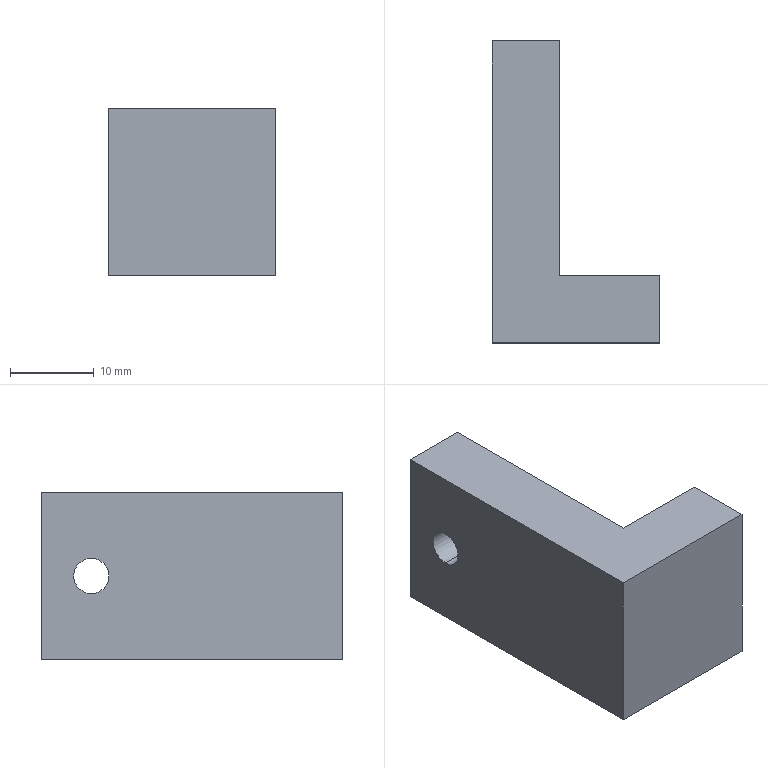Part | SolidWorks | features 3DProfileFeature 1, Extrusion 1, HoleWzd 1 | 1 solid | 10 faces | box 20 x 36 x 20 mm | volume 7569 mm3 | plane 8 | cylinder 2 | commonest cylinder face diameters 4.2 x2
STEP:
#1=CARTESIAN_POINT('',(-12.,30.,-2.1));
#2=VERTEX_POINT('',#1);
#3=CARTESIAN_POINT('',(-12.,30.,2.1));
#4=VERTEX_POINT('',#3);
#5=CARTESIAN_POINT('',(-12.,30.,0.));
#6=DIRECTION('',(-1.,0.,0.));
#7=DIRECTION('',(0.,0.,1.));
#8=AXIS2_PLACEMENT_3D('',#5,#6,#7);
#9=CIRCLE('',#8,2.1);
#10=EDGE_CURVE('',#2,#4,#9,.T.);
#11=ORIENTED_EDGE('',*,*,#10,.F.);
#12=CARTESIAN_POINT('',(-20.,30.,-2.1));
#13=VERTEX_POINT('',#12);
#14=CARTESIAN_POINT('',(-20.,30.,-2.1));
#15=DIRECTION('',(-1.,0.,0.));
#16=VECTOR('',#15,1000.);
#17=LINE('',#14,#16);
#18=EDGE_CURVE('',#2,#13,#17,.T.);
#19=ORIENTED_EDGE('',*,*,#18,.T.);
#20=CARTESIAN_POINT('',(-20.,30.,2.1));
#21=VERTEX_POINT('',#20);
#22=CARTESIAN_POINT('',(-20.,30.,0.));
#23=DIRECTION('',(-1.,0.,0.));
#24=DIRECTION('',(0.,0.,1.));
#25=AXIS2_PLACEMENT_3D('',#22,#23,#24);
#26=CIRCLE('',#25,2.1);
#27=EDGE_CURVE('',#13,#21,#26,.T.);
#28=ORIENTED_EDGE('',*,*,#27,.T.);
#29=CARTESIAN_POINT('',(-20.,30.,2.1));
#30=DIRECTION('',(-1.,0.,0.));
#31=VECTOR('',#30,1000.);
#32=LINE('',#29,#31);
#33=EDGE_CURVE('',#4,#21,#32,.T.);
#34=ORIENTED_EDGE('',*,*,#33,.F.);
#35=EDGE_LOOP('',(#11,#19,#28,#34));
#36=FACE_OUTER_BOUND('',#35,.T.);
#37=CARTESIAN_POINT('',(-20.,30.,0.));
#38=DIRECTION('',(-1.,0.,0.));
#39=DIRECTION('',(0.,0.,1.));
#40=AXIS2_PLACEMENT_3D('',#37,#38,#39);
#41=CYLINDRICAL_SURFACE('',#40,2.1);
#42=ADVANCED_FACE('',(#36),#41,.F.);
#43=CARTESIAN_POINT('',(-20.,36.,-10.));
#44=VERTEX_POINT('',#43);
#45=CARTESIAN_POINT('',(-20.,0.,-10.));
#46=VERTEX_POINT('',#45);
#47=CARTESIAN_POINT('',(-20.,0.,-10.));
#48=DIRECTION('',(0.,-1.,0.));
#49=VECTOR('',#48,1000.);
#50=LINE('',#47,#49);
#51=EDGE_CURVE('',#44,#46,#50,.T.);
#52=ORIENTED_EDGE('',*,*,#51,.T.);
#53=CARTESIAN_POINT('',(-20.,0.,10.));
#54=VERTEX_POINT('',#53);
#55=CARTESIAN_POINT('',(-20.,0.,10.));
#56=DIRECTION('',(0.,0.,-1.));
#57=VECTOR('',#56,1000.);
#58=LINE('',#55,#57);
#59=EDGE_CURVE('',#54,#46,#58,.T.);
#60=ORIENTED_EDGE('',*,*,#59,.F.);
#61=CARTESIAN_POINT('',(-20.,36.,10.));
#62=VERTEX_POINT('',#61);
#63=CARTESIAN_POINT('',(-20.,0.,10.));
#64=DIRECTION('',(0.,-1.,0.));
#65=VECTOR('',#64,1000.);
#66=LINE('',#63,#65);
#67=EDGE_CURVE('',#62,#54,#66,.T.);
#68=ORIENTED_EDGE('',*,*,#67,.F.);
#69=CARTESIAN_POINT('',(-20.,36.,10.));
#70=DIRECTION('',(0.,0.,-1.));
#71=VECTOR('',#70,1000.);
#72=LINE('',#69,#71);
#73=EDGE_CURVE('',#62,#44,#72,.T.);
#74=ORIENTED_EDGE('',*,*,#73,.T.);
#75=EDGE_LOOP('',(#52,#60,#68,#74));
#76=FACE_OUTER_BOUND('',#75,.T.);
#77=CARTESIAN_POINT('',(-20.,30.,0.));
#78=DIRECTION('',(-1.,0.,0.));
#79=DIRECTION('',(0.,0.,1.));
#80=AXIS2_PLACEMENT_3D('',#77,#78,#79);
#81=CIRCLE('',#80,2.1);
#82=EDGE_CURVE('',#21,#13,#81,.T.);
#83=ORIENTED_EDGE('',*,*,#82,.F.);
#84=ORIENTED_EDGE('',*,*,#27,.F.);
#85=EDGE_LOOP('',(#83,#84));
#86=FACE_BOUND('',#85,.T.);
#87=CARTESIAN_POINT('',(-20.,0.,10.));
#88=DIRECTION('',(1.,0.,0.));
#89=DIRECTION('',(0.,0.,-1.));
#90=AXIS2_PLACEMENT_3D('',#87,#88,#89);
#91=PLANE('',#90);
#92=ADVANCED_FACE('',(#76,#86),#91,.F.);
#93=CARTESIAN_POINT('',(0.,0.,-10.));
#94=VERTEX_POINT('',#93);
#95=CARTESIAN_POINT('',(0.,8.,-10.));
#96=VERTEX_POINT('',#95);
#97=CARTESIAN_POINT('',(0.,8.,-10.));
#98=DIRECTION('',(0.,1.,0.));
#99=VECTOR('',#98,1000.);
#100=LINE('',#97,#99);
#101=EDGE_CURVE('',#94,#96,#100,.T.);
#102=ORIENTED_EDGE('',*,*,#101,.T.);
#103=CARTESIAN_POINT('',(0.,8.,10.));
#104=VERTEX_POINT('',#103);
#105=CARTESIAN_POINT('',(0.,8.,10.));
#106=DIRECTION('',(0.,0.,-1.));
#107=VECTOR('',#106,1000.);
#108=LINE('',#105,#107);
#109=EDGE_CURVE('',#104,#96,#108,.T.);
#110=ORIENTED_EDGE('',*,*,#109,.F.);
#111=CARTESIAN_POINT('',(0.,0.,10.));
#112=VERTEX_POINT('',#111);
#113=CARTESIAN_POINT('',(0.,8.,10.));
#114=DIRECTION('',(0.,1.,0.));
#115=VECTOR('',#114,1000.);
#116=LINE('',#113,#115);
#117=EDGE_CURVE('',#112,#104,#116,.T.);
#118=ORIENTED_EDGE('',*,*,#117,.F.);
#119=CARTESIAN_POINT('',(0.,0.,10.));
#120=DIRECTION('',(0.,0.,-1.));
#121=VECTOR('',#120,1000.);
#122=LINE('',#119,#121);
#123=EDGE_CURVE('',#112,#94,#122,.T.);
#124=ORIENTED_EDGE('',*,*,#123,.T.);
#125=EDGE_LOOP('',(#102,#110,#118,#124));
#126=FACE_OUTER_BOUND('',#125,.T.);
#127=CARTESIAN_POINT('',(0.,8.,10.));
#128=DIRECTION('',(-1.,0.,0.));
#129=DIRECTION('',(0.,-1.,0.));
#130=AXIS2_PLACEMENT_3D('',#127,#128,#129);
#131=PLANE('',#130);
#132=ADVANCED_FACE('',(#126),#131,.F.);
#133=CARTESIAN_POINT('',(-12.,8.,-10.));
#134=VERTEX_POINT('',#133);
#135=CARTESIAN_POINT('',(-12.,8.,-10.));
#136=DIRECTION('',(-1.,0.,0.));
#137=VECTOR('',#136,1000.);
#138=LINE('',#135,#137);
#139=EDGE_CURVE('',#96,#134,#138,.T.);
#140=ORIENTED_EDGE('',*,*,#139,.T.);
#141=CARTESIAN_POINT('',(-12.,8.,10.));
#142=VERTEX_POINT('',#141);
#143=CARTESIAN_POINT('',(-12.,8.,10.));
#144=DIRECTION('',(0.,0.,-1.));
#145=VECTOR('',#144,1000.);
#146=LINE('',#143,#145);
#147=EDGE_CURVE('',#142,#134,#146,.T.);
#148=ORIENTED_EDGE('',*,*,#147,.F.);
#149=CARTESIAN_POINT('',(-12.,8.,10.));
#150=DIRECTION('',(-1.,0.,0.));
#151=VECTOR('',#150,1000.);
#152=LINE('',#149,#151);
#153=EDGE_CURVE('',#104,#142,#152,.T.);
#154=ORIENTED_EDGE('',*,*,#153,.F.);
#155=ORIENTED_EDGE('',*,*,#109,.T.);
#156=EDGE_LOOP('',(#140,#148,#154,#155));
#157=FACE_OUTER_BOUND('',#156,.T.);
#158=CARTESIAN_POINT('',(-12.,8.,10.));
#159=DIRECTION('',(0.,-1.,0.));
#160=DIRECTION('',(0.,0.,-1.));
#161=AXIS2_PLACEMENT_3D('',#158,#159,#160);
#162=PLANE('',#161);
#163=ADVANCED_FACE('',(#157),#162,.F.);
#164=CARTESIAN_POINT('',(-12.,30.,0.));
#165=DIRECTION('',(-1.,0.,0.));
#166=DIRECTION('',(0.,0.,1.));
#167=AXIS2_PLACEMENT_3D('',#164,#165,#166);
#168=CIRCLE('',#167,2.1);
#169=EDGE_CURVE('',#4,#2,#168,.T.);
#170=ORIENTED_EDGE('',*,*,#169,.T.);
#171=ORIENTED_EDGE('',*,*,#10,.T.);
#172=EDGE_LOOP('',(#170,#171));
#173=FACE_BOUND('',#172,.T.);
#174=CARTESIAN_POINT('',(-12.,36.,-10.));
#175=VERTEX_POINT('',#174);
#176=CARTESIAN_POINT('',(-12.,36.,-10.));
#177=DIRECTION('',(0.,1.,0.));
#178=VECTOR('',#177,1000.);
#179=LINE('',#176,#178);
#180=EDGE_CURVE('',#134,#175,#179,.T.);
#181=ORIENTED_EDGE('',*,*,#180,.T.);
#182=CARTESIAN_POINT('',(-12.,36.,10.));
#183=VERTEX_POINT('',#182);
#184=CARTESIAN_POINT('',(-12.,36.,10.));
#185=DIRECTION('',(0.,0.,-1.));
#186=VECTOR('',#185,1000.);
#187=LINE('',#184,#186);
#188=EDGE_CURVE('',#183,#175,#187,.T.);
#189=ORIENTED_EDGE('',*,*,#188,.F.);
#190=CARTESIAN_POINT('',(-12.,36.,10.));
#191=DIRECTION('',(0.,1.,0.));
#192=VECTOR('',#191,1000.);
#193=LINE('',#190,#192);
#194=EDGE_CURVE('',#142,#183,#193,.T.);
#195=ORIENTED_EDGE('',*,*,#194,.F.);
#196=ORIENTED_EDGE('',*,*,#147,.T.);
#197=EDGE_LOOP('',(#181,#189,#195,#196));
#198=FACE_OUTER_BOUND('',#197,.T.);
#199=CARTESIAN_POINT('',(-12.,36.,10.));
#200=DIRECTION('',(-1.,0.,0.));
#201=DIRECTION('',(0.,0.,1.));
#202=AXIS2_PLACEMENT_3D('',#199,#200,#201);
#203=PLANE('',#202);
#204=ADVANCED_FACE('',(#173,#198),#203,.F.);
#205=CARTESIAN_POINT('',(-20.,36.,-10.));
#206=DIRECTION('',(-1.,0.,0.));
#207=VECTOR('',#206,1000.);
#208=LINE('',#205,#207);
#209=EDGE_CURVE('',#175,#44,#208,.T.);
#210=ORIENTED_EDGE('',*,*,#209,.T.);
#211=ORIENTED_EDGE('',*,*,#73,.F.);
#212=CARTESIAN_POINT('',(-20.,36.,10.));
#213=DIRECTION('',(-1.,0.,0.));
#214=VECTOR('',#213,1000.);
#215=LINE('',#212,#214);
#216=EDGE_CURVE('',#183,#62,#215,.T.);
#217=ORIENTED_EDGE('',*,*,#216,.F.);
#218=ORIENTED_EDGE('',*,*,#188,.T.);
#219=EDGE_LOOP('',(#210,#211,#217,#218));
#220=FACE_OUTER_BOUND('',#219,.T.);
#221=CARTESIAN_POINT('',(-20.,36.,10.));
#222=DIRECTION('',(0.,-1.,0.));
#223=DIRECTION('',(0.,0.,-1.));
#224=AXIS2_PLACEMENT_3D('',#221,#222,#223);
#225=PLANE('',#224);
#226=ADVANCED_FACE('',(#220),#225,.F.);
#227=CARTESIAN_POINT('',(0.,0.,-10.));
#228=DIRECTION('',(1.,0.,0.));
#229=VECTOR('',#228,1000.);
#230=LINE('',#227,#229);
#231=EDGE_CURVE('',#46,#94,#230,.T.);
#232=ORIENTED_EDGE('',*,*,#231,.T.);
#233=ORIENTED_EDGE('',*,*,#123,.F.);
#234=CARTESIAN_POINT('',(0.,0.,10.));
#235=DIRECTION('',(1.,0.,0.));
#236=VECTOR('',#235,1000.);
#237=LINE('',#234,#236);
#238=EDGE_CURVE('',#54,#112,#237,.T.);
#239=ORIENTED_EDGE('',*,*,#238,.F.);
#240=ORIENTED_EDGE('',*,*,#59,.T.);
#241=EDGE_LOOP('',(#232,#233,#239,#240));
#242=FACE_OUTER_BOUND('',#241,.T.);
#243=CARTESIAN_POINT('',(0.,0.,10.));
#244=DIRECTION('',(0.,1.,0.));
#245=DIRECTION('',(-1.,0.,0.));
#246=AXIS2_PLACEMENT_3D('',#243,#244,#245);
#247=PLANE('',#246);
#248=ADVANCED_FACE('',(#242),#247,.F.);
#249=ORIENTED_EDGE('',*,*,#117,.T.);
#250=ORIENTED_EDGE('',*,*,#153,.T.);
#251=ORIENTED_EDGE('',*,*,#194,.T.);
#252=ORIENTED_EDGE('',*,*,#216,.T.);
#253=ORIENTED_EDGE('',*,*,#67,.T.);
#254=ORIENTED_EDGE('',*,*,#238,.T.);
#255=EDGE_LOOP('',(#249,#250,#251,#252,#253,#254));
#256=FACE_OUTER_BOUND('',#255,.T.);
#257=CARTESIAN_POINT('',(0.,0.,10.));
#258=DIRECTION('',(0.,0.,-1.));
#259=DIRECTION('',(-1.,0.,0.));
#260=AXIS2_PLACEMENT_3D('',#257,#258,#259);
#261=PLANE('',#260);
#262=ADVANCED_FACE('',(#256),#261,.F.);
#263=ORIENTED_EDGE('',*,*,#101,.F.);
#264=ORIENTED_EDGE('',*,*,#231,.F.);
#265=ORIENTED_EDGE('',*,*,#51,.F.);
#266=ORIENTED_EDGE('',*,*,#209,.F.);
#267=ORIENTED_EDGE('',*,*,#180,.F.);
#268=ORIENTED_EDGE('',*,*,#139,.F.);
#269=EDGE_LOOP('',(#263,#264,#265,#266,#267,#268));
#270=FACE_OUTER_BOUND('',#269,.T.);
#271=CARTESIAN_POINT('',(0.,0.,-10.));
#272=DIRECTION('',(0.,0.,-1.));
#273=DIRECTION('',(-1.,0.,0.));
#274=AXIS2_PLACEMENT_3D('',#271,#272,#273);
#275=PLANE('',#274);
#276=ADVANCED_FACE('',(#270),#275,.T.);
#277=ORIENTED_EDGE('',*,*,#18,.F.);
#278=ORIENTED_EDGE('',*,*,#169,.F.);
#279=ORIENTED_EDGE('',*,*,#33,.T.);
#280=ORIENTED_EDGE('',*,*,#82,.T.);
#281=EDGE_LOOP('',(#277,#278,#279,#280));
#282=FACE_OUTER_BOUND('',#281,.T.);
#283=CARTESIAN_POINT('',(-20.,30.,0.));
#284=DIRECTION('',(-1.,0.,0.));
#285=DIRECTION('',(0.,0.,1.));
#286=AXIS2_PLACEMENT_3D('',#283,#284,#285);
#287=CYLINDRICAL_SURFACE('',#286,2.1);
#288=ADVANCED_FACE('',(#282),#287,.F.);
#289=CLOSED_SHELL('',(#42,#92,#132,#163,#204,#226,#248,#262,#276,#288));
#290=MANIFOLD_SOLID_BREP('',#289);
#291=CARTESIAN_POINT('',(0.,0.,0.));
#292=DIRECTION('',(0.,0.,1.));
#293=DIRECTION('',(1.,0.,0.));
#294=AXIS2_PLACEMENT_3D('',#291,#292,#293);
#295=(LENGTH_UNIT()NAMED_UNIT(*)SI_UNIT(.MILLI.,.METRE.));
#296=UNCERTAINTY_MEASURE_WITH_UNIT(LENGTH_MEASURE(0.00001),#295,'','');
#297=(NAMED_UNIT(*)PLANE_ANGLE_UNIT()SI_UNIT($,.RADIAN.));
#298=(NAMED_UNIT(*)SI_UNIT($,.STERADIAN.)SOLID_ANGLE_UNIT());
#299=(GEOMETRIC_REPRESENTATION_CONTEXT(3)GLOBAL_UNCERTAINTY_ASSIGNED_CONTEXT((#296))GLOBAL_UNIT_ASSIGNED_CONTEXT((#295,#297,#298))REPRESENTATION_CONTEXT('',''));
#300=ADVANCED_BREP_SHAPE_REPRESENTATION('',(#290,#294),#299);